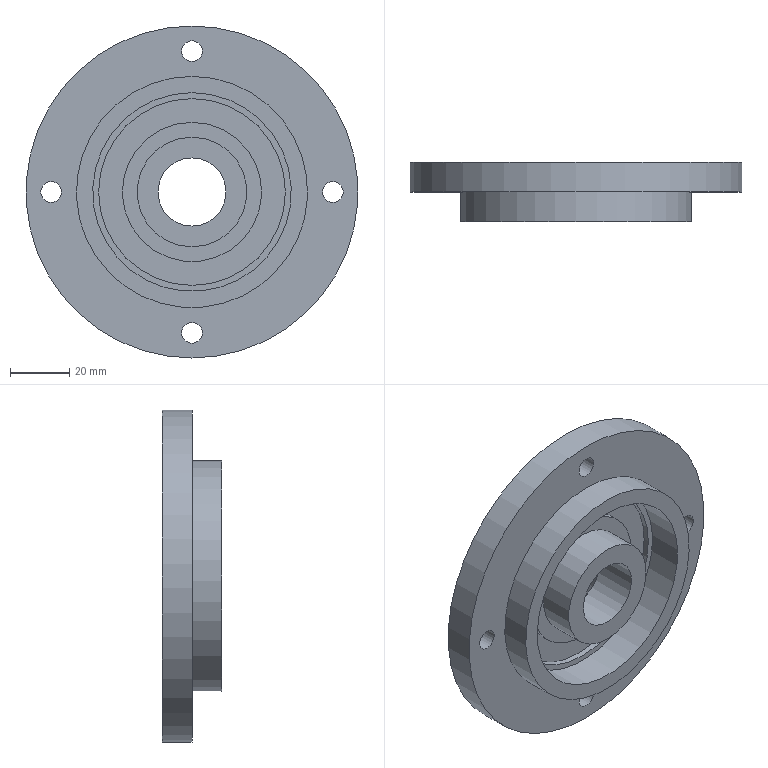Part | STEP file | Outer part of clamping device | 1 solid | 27 faces | box 112 x 20 x 112 mm | volume 101943 mm3 | cylinder 15 | plane 11 | cone 1 | commonest cylinder face diameters 7 x4 12 x4 23 x1 37 x1 47 x1 63 x1
STEP:
#1=CARTESIAN_POINT('',(0.,20.,56.));
#2=VERTEX_POINT('',#1);
#3=CARTESIAN_POINT('',(0.,20.,0.));
#4=DIRECTION('',(0.,1.,0.));
#5=DIRECTION('',(0.,0.,1.));
#6=AXIS2_PLACEMENT_3D('',#3,#4,#5);
#7=CIRCLE('',#6,56.);
#8=EDGE_CURVE('',#2,#2,#7,.T.);
#9=ORIENTED_EDGE('',*,*,#8,.T.);
#10=EDGE_LOOP('',(#9));
#11=FACE_BOUND('',#10,.T.);
#12=CARTESIAN_POINT('',(47.5,20.,6.));
#13=VERTEX_POINT('',#12);
#14=CARTESIAN_POINT('',(47.5,20.,0.));
#15=DIRECTION('',(0.,1.,0.));
#16=DIRECTION('',(0.,0.,1.));
#17=AXIS2_PLACEMENT_3D('',#14,#15,#16);
#18=CIRCLE('',#17,6.);
#19=EDGE_CURVE('',#13,#13,#18,.F.);
#20=ORIENTED_EDGE('',*,*,#19,.T.);
#21=EDGE_LOOP('',(#20));
#22=FACE_BOUND('',#21,.T.);
#23=CARTESIAN_POINT('',(-6.,20.,47.5));
#24=VERTEX_POINT('',#23);
#25=CARTESIAN_POINT('',(0.,20.,47.5));
#26=DIRECTION('',(0.,1.,0.));
#27=DIRECTION('',(-1.,0.,0.));
#28=AXIS2_PLACEMENT_3D('',#25,#26,#27);
#29=CIRCLE('',#28,6.);
#30=EDGE_CURVE('',#24,#24,#29,.F.);
#31=ORIENTED_EDGE('',*,*,#30,.T.);
#32=EDGE_LOOP('',(#31));
#33=FACE_BOUND('',#32,.T.);
#34=CARTESIAN_POINT('',(-47.5,20.,-6.));
#35=VERTEX_POINT('',#34);
#36=CARTESIAN_POINT('',(-47.5,20.,0.));
#37=DIRECTION('',(0.,1.,0.));
#38=DIRECTION('',(0.,0.,-1.));
#39=AXIS2_PLACEMENT_3D('',#36,#37,#38);
#40=CIRCLE('',#39,6.);
#41=EDGE_CURVE('',#35,#35,#40,.F.);
#42=ORIENTED_EDGE('',*,*,#41,.T.);
#43=EDGE_LOOP('',(#42));
#44=FACE_BOUND('',#43,.T.);
#45=CARTESIAN_POINT('',(0.,20.,-15.695));
#46=VERTEX_POINT('',#45);
#47=CARTESIAN_POINT('',(0.,20.,0.));
#48=DIRECTION('',(0.,1.,0.));
#49=DIRECTION('',(0.,0.,-1.));
#50=AXIS2_PLACEMENT_3D('',#47,#48,#49);
#51=CIRCLE('',#50,15.695);
#52=EDGE_CURVE('',#46,#46,#51,.F.);
#53=ORIENTED_EDGE('',*,*,#52,.T.);
#54=EDGE_LOOP('',(#53));
#55=FACE_BOUND('',#54,.T.);
#56=CARTESIAN_POINT('',(6.,20.,-47.5));
#57=VERTEX_POINT('',#56);
#58=CARTESIAN_POINT('',(0.,20.,-47.5));
#59=DIRECTION('',(0.,1.,0.));
#60=DIRECTION('',(1.,0.,0.));
#61=AXIS2_PLACEMENT_3D('',#58,#59,#60);
#62=CIRCLE('',#61,6.);
#63=EDGE_CURVE('',#57,#57,#62,.F.);
#64=ORIENTED_EDGE('',*,*,#63,.T.);
#65=EDGE_LOOP('',(#64));
#66=FACE_BOUND('',#65,.T.);
#67=CARTESIAN_POINT('',(0.,20.,0.));
#68=DIRECTION('',(0.,1.,0.));
#69=DIRECTION('',(0.,0.,1.));
#70=AXIS2_PLACEMENT_3D('',#67,#68,#69);
#71=PLANE('',#70);
#72=ADVANCED_FACE('',(#11,#22,#33,#44,#55,#66),#71,.T.);
#73=CARTESIAN_POINT('',(0.,10.,56.));
#74=VERTEX_POINT('',#73);
#75=CARTESIAN_POINT('',(0.,10.,0.));
#76=DIRECTION('',(0.,1.,0.));
#77=DIRECTION('',(0.,0.,1.));
#78=AXIS2_PLACEMENT_3D('',#75,#76,#77);
#79=CIRCLE('',#78,56.);
#80=EDGE_CURVE('',#74,#74,#79,.T.);
#81=ORIENTED_EDGE('',*,*,#80,.F.);
#82=EDGE_LOOP('',(#81));
#83=FACE_BOUND('',#82,.T.);
#84=CARTESIAN_POINT('',(47.5,10.,3.5));
#85=VERTEX_POINT('',#84);
#86=CARTESIAN_POINT('',(47.5,10.,0.));
#87=DIRECTION('',(0.,1.,0.));
#88=DIRECTION('',(0.,0.,1.));
#89=AXIS2_PLACEMENT_3D('',#86,#87,#88);
#90=CIRCLE('',#89,3.5);
#91=EDGE_CURVE('',#85,#85,#90,.T.);
#92=ORIENTED_EDGE('',*,*,#91,.T.);
#93=EDGE_LOOP('',(#92));
#94=FACE_BOUND('',#93,.T.);
#95=CARTESIAN_POINT('',(-3.5,10.,47.5));
#96=VERTEX_POINT('',#95);
#97=CARTESIAN_POINT('',(0.,10.,47.5));
#98=DIRECTION('',(0.,1.,0.));
#99=DIRECTION('',(-1.,0.,0.));
#100=AXIS2_PLACEMENT_3D('',#97,#98,#99);
#101=CIRCLE('',#100,3.5);
#102=EDGE_CURVE('',#96,#96,#101,.T.);
#103=ORIENTED_EDGE('',*,*,#102,.T.);
#104=EDGE_LOOP('',(#103));
#105=FACE_BOUND('',#104,.T.);
#106=CARTESIAN_POINT('',(-47.5,10.,-3.5));
#107=VERTEX_POINT('',#106);
#108=CARTESIAN_POINT('',(-47.5,10.,0.));
#109=DIRECTION('',(0.,1.,0.));
#110=DIRECTION('',(0.,0.,-1.));
#111=AXIS2_PLACEMENT_3D('',#108,#109,#110);
#112=CIRCLE('',#111,3.5);
#113=EDGE_CURVE('',#107,#107,#112,.T.);
#114=ORIENTED_EDGE('',*,*,#113,.T.);
#115=EDGE_LOOP('',(#114));
#116=FACE_BOUND('',#115,.T.);
#117=CARTESIAN_POINT('',(0.,10.,39.));
#118=VERTEX_POINT('',#117);
#119=CARTESIAN_POINT('',(0.,10.,0.));
#120=DIRECTION('',(0.,1.,0.));
#121=DIRECTION('',(0.,0.,1.));
#122=AXIS2_PLACEMENT_3D('',#119,#120,#121);
#123=CIRCLE('',#122,39.);
#124=EDGE_CURVE('',#118,#118,#123,.T.);
#125=ORIENTED_EDGE('',*,*,#124,.T.);
#126=EDGE_LOOP('',(#125));
#127=FACE_BOUND('',#126,.T.);
#128=CARTESIAN_POINT('',(3.5,10.,-47.5));
#129=VERTEX_POINT('',#128);
#130=CARTESIAN_POINT('',(0.,10.,-47.5));
#131=DIRECTION('',(0.,1.,0.));
#132=DIRECTION('',(1.,0.,0.));
#133=AXIS2_PLACEMENT_3D('',#130,#131,#132);
#134=CIRCLE('',#133,3.5);
#135=EDGE_CURVE('',#129,#129,#134,.T.);
#136=ORIENTED_EDGE('',*,*,#135,.T.);
#137=EDGE_LOOP('',(#136));
#138=FACE_BOUND('',#137,.T.);
#139=CARTESIAN_POINT('',(0.,10.,0.));
#140=DIRECTION('',(0.,-1.,0.));
#141=DIRECTION('',(0.,0.,1.));
#142=AXIS2_PLACEMENT_3D('',#139,#140,#141);
#143=PLANE('',#142);
#144=ADVANCED_FACE('',(#83,#94,#105,#116,#127,#138),#143,.T.);
#145=CARTESIAN_POINT('',(-47.5,15.,-3.5));
#146=VERTEX_POINT('',#145);
#147=CARTESIAN_POINT('',(-47.5,15.,0.));
#148=DIRECTION('',(0.,1.,0.));
#149=DIRECTION('',(0.,0.,-1.));
#150=AXIS2_PLACEMENT_3D('',#147,#148,#149);
#151=CIRCLE('',#150,3.5);
#152=EDGE_CURVE('',#146,#146,#151,.T.);
#153=ORIENTED_EDGE('',*,*,#152,.T.);
#154=EDGE_LOOP('',(#153));
#155=FACE_OUTER_BOUND('',#154,.T.);
#156=ORIENTED_EDGE('',*,*,#113,.F.);
#157=EDGE_LOOP('',(#156));
#158=FACE_OUTER_BOUND('',#157,.T.);
#159=CARTESIAN_POINT('',(-47.5,-20.,0.));
#160=DIRECTION('',(0.,1.,0.));
#161=DIRECTION('',(0.,0.,-1.));
#162=AXIS2_PLACEMENT_3D('',#159,#160,#161);
#163=CYLINDRICAL_SURFACE('',#162,3.5);
#164=ADVANCED_FACE('',(#155,#158),#163,.F.);
#165=ORIENTED_EDGE('',*,*,#41,.F.);
#166=EDGE_LOOP('',(#165));
#167=FACE_OUTER_BOUND('',#166,.T.);
#168=CARTESIAN_POINT('',(-47.5,15.,-6.));
#169=VERTEX_POINT('',#168);
#170=CARTESIAN_POINT('',(-47.5,15.,0.));
#171=DIRECTION('',(0.,1.,0.));
#172=DIRECTION('',(0.,0.,-1.));
#173=AXIS2_PLACEMENT_3D('',#170,#171,#172);
#174=CIRCLE('',#173,6.);
#175=EDGE_CURVE('',#169,#169,#174,.T.);
#176=ORIENTED_EDGE('',*,*,#175,.F.);
#177=EDGE_LOOP('',(#176));
#178=FACE_OUTER_BOUND('',#177,.T.);
#179=CARTESIAN_POINT('',(-47.5,15.,0.));
#180=DIRECTION('',(0.,1.,0.));
#181=DIRECTION('',(0.,0.,-1.));
#182=AXIS2_PLACEMENT_3D('',#179,#180,#181);
#183=CYLINDRICAL_SURFACE('',#182,6.);
#184=ADVANCED_FACE('',(#167,#178),#183,.F.);
#185=CARTESIAN_POINT('',(-3.5,15.,47.5));
#186=VERTEX_POINT('',#185);
#187=CARTESIAN_POINT('',(0.,15.,47.5));
#188=DIRECTION('',(0.,1.,0.));
#189=DIRECTION('',(-1.,0.,0.));
#190=AXIS2_PLACEMENT_3D('',#187,#188,#189);
#191=CIRCLE('',#190,3.5);
#192=EDGE_CURVE('',#186,#186,#191,.T.);
#193=ORIENTED_EDGE('',*,*,#192,.T.);
#194=EDGE_LOOP('',(#193));
#195=FACE_OUTER_BOUND('',#194,.T.);
#196=ORIENTED_EDGE('',*,*,#102,.F.);
#197=EDGE_LOOP('',(#196));
#198=FACE_OUTER_BOUND('',#197,.T.);
#199=CARTESIAN_POINT('',(0.,-20.,47.5));
#200=DIRECTION('',(0.,1.,0.));
#201=DIRECTION('',(-1.,0.,0.));
#202=AXIS2_PLACEMENT_3D('',#199,#200,#201);
#203=CYLINDRICAL_SURFACE('',#202,3.5);
#204=ADVANCED_FACE('',(#195,#198),#203,.F.);
#205=ORIENTED_EDGE('',*,*,#30,.F.);
#206=EDGE_LOOP('',(#205));
#207=FACE_OUTER_BOUND('',#206,.T.);
#208=CARTESIAN_POINT('',(-6.,15.,47.5));
#209=VERTEX_POINT('',#208);
#210=CARTESIAN_POINT('',(0.,15.,47.5));
#211=DIRECTION('',(0.,1.,0.));
#212=DIRECTION('',(-1.,0.,0.));
#213=AXIS2_PLACEMENT_3D('',#210,#211,#212);
#214=CIRCLE('',#213,6.);
#215=EDGE_CURVE('',#209,#209,#214,.T.);
#216=ORIENTED_EDGE('',*,*,#215,.F.);
#217=EDGE_LOOP('',(#216));
#218=FACE_OUTER_BOUND('',#217,.T.);
#219=CARTESIAN_POINT('',(0.,15.,47.5));
#220=DIRECTION('',(0.,1.,0.));
#221=DIRECTION('',(-1.,0.,0.));
#222=AXIS2_PLACEMENT_3D('',#219,#220,#221);
#223=CYLINDRICAL_SURFACE('',#222,6.);
#224=ADVANCED_FACE('',(#207,#218),#223,.F.);
#225=CARTESIAN_POINT('',(47.5,15.,3.5));
#226=VERTEX_POINT('',#225);
#227=CARTESIAN_POINT('',(47.5,15.,0.));
#228=DIRECTION('',(0.,1.,0.));
#229=DIRECTION('',(0.,0.,1.));
#230=AXIS2_PLACEMENT_3D('',#227,#228,#229);
#231=CIRCLE('',#230,3.5);
#232=EDGE_CURVE('',#226,#226,#231,.T.);
#233=ORIENTED_EDGE('',*,*,#232,.T.);
#234=EDGE_LOOP('',(#233));
#235=FACE_OUTER_BOUND('',#234,.T.);
#236=ORIENTED_EDGE('',*,*,#91,.F.);
#237=EDGE_LOOP('',(#236));
#238=FACE_OUTER_BOUND('',#237,.T.);
#239=CARTESIAN_POINT('',(47.5,-20.,0.));
#240=DIRECTION('',(0.,1.,0.));
#241=DIRECTION('',(0.,0.,1.));
#242=AXIS2_PLACEMENT_3D('',#239,#240,#241);
#243=CYLINDRICAL_SURFACE('',#242,3.5);
#244=ADVANCED_FACE('',(#235,#238),#243,.F.);
#245=ORIENTED_EDGE('',*,*,#19,.F.);
#246=EDGE_LOOP('',(#245));
#247=FACE_OUTER_BOUND('',#246,.T.);
#248=CARTESIAN_POINT('',(47.5,15.,6.));
#249=VERTEX_POINT('',#248);
#250=CARTESIAN_POINT('',(47.5,15.,0.));
#251=DIRECTION('',(0.,1.,0.));
#252=DIRECTION('',(0.,0.,1.));
#253=AXIS2_PLACEMENT_3D('',#250,#251,#252);
#254=CIRCLE('',#253,6.);
#255=EDGE_CURVE('',#249,#249,#254,.T.);
#256=ORIENTED_EDGE('',*,*,#255,.F.);
#257=EDGE_LOOP('',(#256));
#258=FACE_OUTER_BOUND('',#257,.T.);
#259=CARTESIAN_POINT('',(47.5,15.,0.));
#260=DIRECTION('',(0.,1.,0.));
#261=DIRECTION('',(0.,0.,1.));
#262=AXIS2_PLACEMENT_3D('',#259,#260,#261);
#263=CYLINDRICAL_SURFACE('',#262,6.);
#264=ADVANCED_FACE('',(#247,#258),#263,.F.);
#265=ORIENTED_EDGE('',*,*,#8,.F.);
#266=EDGE_LOOP('',(#265));
#267=FACE_OUTER_BOUND('',#266,.T.);
#268=ORIENTED_EDGE('',*,*,#80,.T.);
#269=EDGE_LOOP('',(#268));
#270=FACE_OUTER_BOUND('',#269,.T.);
#271=CARTESIAN_POINT('',(0.,10.,0.));
#272=DIRECTION('',(0.,1.,0.));
#273=DIRECTION('',(0.,0.,1.));
#274=AXIS2_PLACEMENT_3D('',#271,#272,#273);
#275=CYLINDRICAL_SURFACE('',#274,56.);
#276=ADVANCED_FACE('',(#267,#270),#275,.T.);
#277=ORIENTED_EDGE('',*,*,#52,.F.);
#278=EDGE_LOOP('',(#277));
#279=FACE_OUTER_BOUND('',#278,.T.);
#280=CARTESIAN_POINT('',(0.,15.,-11.5));
#281=VERTEX_POINT('',#280);
#282=CARTESIAN_POINT('',(0.,15.,11.5));
#283=VERTEX_POINT('',#282);
#284=CARTESIAN_POINT('',(0.,15.,0.));
#285=DIRECTION('',(0.,1.,0.));
#286=DIRECTION('',(0.,0.,-1.));
#287=AXIS2_PLACEMENT_3D('',#284,#285,#286);
#288=CIRCLE('',#287,11.5);
#289=EDGE_CURVE('',#281,#283,#288,.T.);
#290=ORIENTED_EDGE('',*,*,#289,.F.);
#291=CARTESIAN_POINT('',(0.,15.,0.));
#292=DIRECTION('',(0.,1.,0.));
#293=DIRECTION('',(0.,0.,1.));
#294=AXIS2_PLACEMENT_3D('',#291,#292,#293);
#295=CIRCLE('',#294,11.5);
#296=EDGE_CURVE('',#283,#281,#295,.T.);
#297=ORIENTED_EDGE('',*,*,#296,.F.);
#298=EDGE_LOOP('',(#290,#297));
#299=FACE_BOUND('',#298,.T.);
#300=CARTESIAN_POINT('',(0.,17.5,0.));
#301=DIRECTION('',(0.,1.,0.));
#302=DIRECTION('',(0.,0.,-1.));
#303=AXIS2_PLACEMENT_3D('',#300,#301,#302);
#304=CONICAL_SURFACE('',#303,13.598,0.6981);
#305=ADVANCED_FACE('',(#279,#299),#304,.F.);
#306=ORIENTED_EDGE('',*,*,#63,.F.);
#307=EDGE_LOOP('',(#306));
#308=FACE_OUTER_BOUND('',#307,.T.);
#309=CARTESIAN_POINT('',(6.,15.,-47.5));
#310=VERTEX_POINT('',#309);
#311=CARTESIAN_POINT('',(0.,15.,-47.5));
#312=DIRECTION('',(0.,1.,0.));
#313=DIRECTION('',(1.,0.,0.));
#314=AXIS2_PLACEMENT_3D('',#311,#312,#313);
#315=CIRCLE('',#314,6.);
#316=EDGE_CURVE('',#310,#310,#315,.T.);
#317=ORIENTED_EDGE('',*,*,#316,.F.);
#318=EDGE_LOOP('',(#317));
#319=FACE_OUTER_BOUND('',#318,.T.);
#320=CARTESIAN_POINT('',(0.,15.,-47.5));
#321=DIRECTION('',(0.,1.,0.));
#322=DIRECTION('',(1.,0.,0.));
#323=AXIS2_PLACEMENT_3D('',#320,#321,#322);
#324=CYLINDRICAL_SURFACE('',#323,6.);
#325=ADVANCED_FACE('',(#308,#319),#324,.F.);
#326=ORIENTED_EDGE('',*,*,#124,.F.);
#327=EDGE_LOOP('',(#326));
#328=FACE_OUTER_BOUND('',#327,.T.);
#329=CARTESIAN_POINT('',(0.,0.,39.));
#330=VERTEX_POINT('',#329);
#331=CARTESIAN_POINT('',(0.,0.,0.));
#332=DIRECTION('',(0.,1.,0.));
#333=DIRECTION('',(0.,0.,1.));
#334=AXIS2_PLACEMENT_3D('',#331,#332,#333);
#335=CIRCLE('',#334,39.);
#336=EDGE_CURVE('',#330,#330,#335,.T.);
#337=ORIENTED_EDGE('',*,*,#336,.T.);
#338=EDGE_LOOP('',(#337));
#339=FACE_OUTER_BOUND('',#338,.T.);
#340=CARTESIAN_POINT('',(0.,0.,0.));
#341=DIRECTION('',(0.,1.,0.));
#342=DIRECTION('',(0.,0.,1.));
#343=AXIS2_PLACEMENT_3D('',#340,#341,#342);
#344=CYLINDRICAL_SURFACE('',#343,39.);
#345=ADVANCED_FACE('',(#328,#339),#344,.T.);
#346=CARTESIAN_POINT('',(3.5,15.,-47.5));
#347=VERTEX_POINT('',#346);
#348=CARTESIAN_POINT('',(0.,15.,-47.5));
#349=DIRECTION('',(0.,1.,0.));
#350=DIRECTION('',(1.,0.,0.));
#351=AXIS2_PLACEMENT_3D('',#348,#349,#350);
#352=CIRCLE('',#351,3.5);
#353=EDGE_CURVE('',#347,#347,#352,.T.);
#354=ORIENTED_EDGE('',*,*,#353,.T.);
#355=EDGE_LOOP('',(#354));
#356=FACE_OUTER_BOUND('',#355,.T.);
#357=ORIENTED_EDGE('',*,*,#135,.F.);
#358=EDGE_LOOP('',(#357));
#359=FACE_OUTER_BOUND('',#358,.T.);
#360=CARTESIAN_POINT('',(0.,-20.,-47.5));
#361=DIRECTION('',(0.,1.,0.));
#362=DIRECTION('',(1.,0.,0.));
#363=AXIS2_PLACEMENT_3D('',#360,#361,#362);
#364=CYLINDRICAL_SURFACE('',#363,3.5);
#365=ADVANCED_FACE('',(#356,#359),#364,.F.);
#366=ORIENTED_EDGE('',*,*,#175,.T.);
#367=EDGE_LOOP('',(#366));
#368=FACE_BOUND('',#367,.T.);
#369=ORIENTED_EDGE('',*,*,#152,.F.);
#370=EDGE_LOOP('',(#369));
#371=FACE_BOUND('',#370,.T.);
#372=CARTESIAN_POINT('',(-47.5,15.,0.));
#373=DIRECTION('',(0.,-1.,0.));
#374=DIRECTION('',(0.,0.,-1.));
#375=AXIS2_PLACEMENT_3D('',#372,#373,#374);
#376=PLANE('',#375);
#377=ADVANCED_FACE('',(#368,#371),#376,.F.);
#378=ORIENTED_EDGE('',*,*,#215,.T.);
#379=EDGE_LOOP('',(#378));
#380=FACE_BOUND('',#379,.T.);
#381=ORIENTED_EDGE('',*,*,#192,.F.);
#382=EDGE_LOOP('',(#381));
#383=FACE_BOUND('',#382,.T.);
#384=CARTESIAN_POINT('',(0.,15.,47.5));
#385=DIRECTION('',(0.,-1.,0.));
#386=DIRECTION('',(-1.,0.,0.));
#387=AXIS2_PLACEMENT_3D('',#384,#385,#386);
#388=PLANE('',#387);
#389=ADVANCED_FACE('',(#380,#383),#388,.F.);
#390=ORIENTED_EDGE('',*,*,#255,.T.);
#391=EDGE_LOOP('',(#390));
#392=FACE_BOUND('',#391,.T.);
#393=ORIENTED_EDGE('',*,*,#232,.F.);
#394=EDGE_LOOP('',(#393));
#395=FACE_BOUND('',#394,.T.);
#396=CARTESIAN_POINT('',(47.5,15.,0.));
#397=DIRECTION('',(0.,-1.,0.));
#398=DIRECTION('',(0.,0.,1.));
#399=AXIS2_PLACEMENT_3D('',#396,#397,#398);
#400=PLANE('',#399);
#401=ADVANCED_FACE('',(#392,#395),#400,.F.);
#402=ORIENTED_EDGE('',*,*,#296,.T.);
#403=ORIENTED_EDGE('',*,*,#289,.T.);
#404=EDGE_LOOP('',(#402,#403));
#405=FACE_BOUND('',#404,.T.);
#406=CARTESIAN_POINT('',(0.,0.,11.5));
#407=VERTEX_POINT('',#406);
#408=CARTESIAN_POINT('',(0.,0.,0.));
#409=DIRECTION('',(0.,1.,0.));
#410=DIRECTION('',(0.,0.,1.));
#411=AXIS2_PLACEMENT_3D('',#408,#409,#410);
#412=CIRCLE('',#411,11.5);
#413=EDGE_CURVE('',#407,#407,#412,.T.);
#414=ORIENTED_EDGE('',*,*,#413,.F.);
#415=EDGE_LOOP('',(#414));
#416=FACE_OUTER_BOUND('',#415,.T.);
#417=CARTESIAN_POINT('',(0.,20.,0.));
#418=DIRECTION('',(0.,1.,0.));
#419=DIRECTION('',(0.,0.,1.));
#420=AXIS2_PLACEMENT_3D('',#417,#418,#419);
#421=CYLINDRICAL_SURFACE('',#420,11.5);
#422=ADVANCED_FACE('',(#405,#416),#421,.F.);
#423=ORIENTED_EDGE('',*,*,#316,.T.);
#424=EDGE_LOOP('',(#423));
#425=FACE_BOUND('',#424,.T.);
#426=ORIENTED_EDGE('',*,*,#353,.F.);
#427=EDGE_LOOP('',(#426));
#428=FACE_BOUND('',#427,.T.);
#429=CARTESIAN_POINT('',(0.,15.,-47.5));
#430=DIRECTION('',(0.,-1.,0.));
#431=DIRECTION('',(1.,0.,0.));
#432=AXIS2_PLACEMENT_3D('',#429,#430,#431);
#433=PLANE('',#432);
#434=ADVANCED_FACE('',(#425,#428),#433,.F.);
#435=ORIENTED_EDGE('',*,*,#336,.F.);
#436=EDGE_LOOP('',(#435));
#437=FACE_BOUND('',#436,.T.);
#438=CARTESIAN_POINT('',(0.,0.,33.5));
#439=VERTEX_POINT('',#438);
#440=CARTESIAN_POINT('',(0.,0.,0.));
#441=DIRECTION('',(0.,1.,0.));
#442=DIRECTION('',(0.,0.,1.));
#443=AXIS2_PLACEMENT_3D('',#440,#441,#442);
#444=CIRCLE('',#443,33.5);
#445=EDGE_CURVE('',#439,#439,#444,.T.);
#446=ORIENTED_EDGE('',*,*,#445,.T.);
#447=EDGE_LOOP('',(#446));
#448=FACE_BOUND('',#447,.T.);
#449=CARTESIAN_POINT('',(0.,0.,0.));
#450=DIRECTION('',(0.,-1.,0.));
#451=DIRECTION('',(0.,0.,1.));
#452=AXIS2_PLACEMENT_3D('',#449,#450,#451);
#453=PLANE('',#452);
#454=ADVANCED_FACE('',(#437,#448),#453,.T.);
#455=CARTESIAN_POINT('',(0.,0.,18.5));
#456=VERTEX_POINT('',#455);
#457=CARTESIAN_POINT('',(0.,0.,0.));
#458=DIRECTION('',(0.,1.,0.));
#459=DIRECTION('',(0.,0.,1.));
#460=AXIS2_PLACEMENT_3D('',#457,#458,#459);
#461=CIRCLE('',#460,18.5);
#462=EDGE_CURVE('',#456,#456,#461,.T.);
#463=ORIENTED_EDGE('',*,*,#462,.F.);
#464=EDGE_LOOP('',(#463));
#465=FACE_BOUND('',#464,.T.);
#466=ORIENTED_EDGE('',*,*,#413,.T.);
#467=EDGE_LOOP('',(#466));
#468=FACE_BOUND('',#467,.T.);
#469=CARTESIAN_POINT('',(0.,0.,0.));
#470=DIRECTION('',(0.,-1.,0.));
#471=DIRECTION('',(0.,0.,1.));
#472=AXIS2_PLACEMENT_3D('',#469,#470,#471);
#473=PLANE('',#472);
#474=ADVANCED_FACE('',(#465,#468),#473,.T.);
#475=CARTESIAN_POINT('',(0.,12.,33.5));
#476=VERTEX_POINT('',#475);
#477=CARTESIAN_POINT('',(0.,12.,0.));
#478=DIRECTION('',(0.,1.,0.));
#479=DIRECTION('',(0.,0.,1.));
#480=AXIS2_PLACEMENT_3D('',#477,#478,#479);
#481=CIRCLE('',#480,33.5);
#482=EDGE_CURVE('',#476,#476,#481,.T.);
#483=ORIENTED_EDGE('',*,*,#482,.T.);
#484=EDGE_LOOP('',(#483));
#485=FACE_OUTER_BOUND('',#484,.T.);
#486=ORIENTED_EDGE('',*,*,#445,.F.);
#487=EDGE_LOOP('',(#486));
#488=FACE_OUTER_BOUND('',#487,.T.);
#489=CARTESIAN_POINT('',(0.,12.,0.));
#490=DIRECTION('',(0.,1.,0.));
#491=DIRECTION('',(0.,0.,1.));
#492=AXIS2_PLACEMENT_3D('',#489,#490,#491);
#493=CYLINDRICAL_SURFACE('',#492,33.5);
#494=ADVANCED_FACE('',(#485,#488),#493,.F.);
#495=CARTESIAN_POINT('',(0.,12.,18.5));
#496=VERTEX_POINT('',#495);
#497=CARTESIAN_POINT('',(0.,12.,0.));
#498=DIRECTION('',(0.,1.,0.));
#499=DIRECTION('',(0.,0.,1.));
#500=AXIS2_PLACEMENT_3D('',#497,#498,#499);
#501=CIRCLE('',#500,18.5);
#502=EDGE_CURVE('',#496,#496,#501,.T.);
#503=ORIENTED_EDGE('',*,*,#502,.F.);
#504=EDGE_LOOP('',(#503));
#505=FACE_OUTER_BOUND('',#504,.T.);
#506=ORIENTED_EDGE('',*,*,#462,.T.);
#507=EDGE_LOOP('',(#506));
#508=FACE_OUTER_BOUND('',#507,.T.);
#509=CARTESIAN_POINT('',(0.,0.,0.));
#510=DIRECTION('',(0.,1.,0.));
#511=DIRECTION('',(0.,0.,1.));
#512=AXIS2_PLACEMENT_3D('',#509,#510,#511);
#513=CYLINDRICAL_SURFACE('',#512,18.5);
#514=ADVANCED_FACE('',(#505,#508),#513,.T.);
#515=ORIENTED_EDGE('',*,*,#482,.F.);
#516=EDGE_LOOP('',(#515));
#517=FACE_BOUND('',#516,.T.);
#518=CARTESIAN_POINT('',(0.,12.,31.5));
#519=VERTEX_POINT('',#518);
#520=CARTESIAN_POINT('',(0.,12.,0.));
#521=DIRECTION('',(0.,1.,0.));
#522=DIRECTION('',(0.,0.,1.));
#523=AXIS2_PLACEMENT_3D('',#520,#521,#522);
#524=CIRCLE('',#523,31.5);
#525=EDGE_CURVE('',#519,#519,#524,.T.);
#526=ORIENTED_EDGE('',*,*,#525,.T.);
#527=EDGE_LOOP('',(#526));
#528=FACE_BOUND('',#527,.T.);
#529=CARTESIAN_POINT('',(0.,12.,0.));
#530=DIRECTION('',(0.,-1.,0.));
#531=DIRECTION('',(0.,0.,1.));
#532=AXIS2_PLACEMENT_3D('',#529,#530,#531);
#533=PLANE('',#532);
#534=ADVANCED_FACE('',(#517,#528),#533,.T.);
#535=CARTESIAN_POINT('',(0.,12.,23.5));
#536=VERTEX_POINT('',#535);
#537=CARTESIAN_POINT('',(0.,12.,0.));
#538=DIRECTION('',(0.,1.,0.));
#539=DIRECTION('',(0.,0.,1.));
#540=AXIS2_PLACEMENT_3D('',#537,#538,#539);
#541=CIRCLE('',#540,23.5);
#542=EDGE_CURVE('',#536,#536,#541,.T.);
#543=ORIENTED_EDGE('',*,*,#542,.F.);
#544=EDGE_LOOP('',(#543));
#545=FACE_BOUND('',#544,.T.);
#546=ORIENTED_EDGE('',*,*,#502,.T.);
#547=EDGE_LOOP('',(#546));
#548=FACE_BOUND('',#547,.T.);
#549=CARTESIAN_POINT('',(0.,12.,0.));
#550=DIRECTION('',(0.,-1.,0.));
#551=DIRECTION('',(0.,0.,1.));
#552=AXIS2_PLACEMENT_3D('',#549,#550,#551);
#553=PLANE('',#552);
#554=ADVANCED_FACE('',(#545,#548),#553,.T.);
#555=CARTESIAN_POINT('',(0.,14.,31.5));
#556=VERTEX_POINT('',#555);
#557=CARTESIAN_POINT('',(0.,14.,0.));
#558=DIRECTION('',(0.,1.,0.));
#559=DIRECTION('',(0.,0.,1.));
#560=AXIS2_PLACEMENT_3D('',#557,#558,#559);
#561=CIRCLE('',#560,31.5);
#562=EDGE_CURVE('',#556,#556,#561,.T.);
#563=ORIENTED_EDGE('',*,*,#562,.T.);
#564=EDGE_LOOP('',(#563));
#565=FACE_OUTER_BOUND('',#564,.T.);
#566=ORIENTED_EDGE('',*,*,#525,.F.);
#567=EDGE_LOOP('',(#566));
#568=FACE_OUTER_BOUND('',#567,.T.);
#569=CARTESIAN_POINT('',(0.,14.,0.));
#570=DIRECTION('',(0.,1.,0.));
#571=DIRECTION('',(0.,0.,1.));
#572=AXIS2_PLACEMENT_3D('',#569,#570,#571);
#573=CYLINDRICAL_SURFACE('',#572,31.5);
#574=ADVANCED_FACE('',(#565,#568),#573,.F.);
#575=CARTESIAN_POINT('',(0.,14.,23.5));
#576=VERTEX_POINT('',#575);
#577=CARTESIAN_POINT('',(0.,14.,0.));
#578=DIRECTION('',(0.,1.,0.));
#579=DIRECTION('',(0.,0.,1.));
#580=AXIS2_PLACEMENT_3D('',#577,#578,#579);
#581=CIRCLE('',#580,23.5);
#582=EDGE_CURVE('',#576,#576,#581,.T.);
#583=ORIENTED_EDGE('',*,*,#582,.F.);
#584=EDGE_LOOP('',(#583));
#585=FACE_OUTER_BOUND('',#584,.T.);
#586=ORIENTED_EDGE('',*,*,#542,.T.);
#587=EDGE_LOOP('',(#586));
#588=FACE_OUTER_BOUND('',#587,.T.);
#589=CARTESIAN_POINT('',(0.,12.,0.));
#590=DIRECTION('',(0.,1.,0.));
#591=DIRECTION('',(0.,0.,1.));
#592=AXIS2_PLACEMENT_3D('',#589,#590,#591);
#593=CYLINDRICAL_SURFACE('',#592,23.5);
#594=ADVANCED_FACE('',(#585,#588),#593,.T.);
#595=ORIENTED_EDGE('',*,*,#562,.F.);
#596=EDGE_LOOP('',(#595));
#597=FACE_BOUND('',#596,.T.);
#598=ORIENTED_EDGE('',*,*,#582,.T.);
#599=EDGE_LOOP('',(#598));
#600=FACE_BOUND('',#599,.T.);
#601=CARTESIAN_POINT('',(0.,14.,0.));
#602=DIRECTION('',(0.,-1.,0.));
#603=DIRECTION('',(0.,0.,1.));
#604=AXIS2_PLACEMENT_3D('',#601,#602,#603);
#605=PLANE('',#604);
#606=ADVANCED_FACE('',(#597,#600),#605,.T.);
#607=CLOSED_SHELL('',(#72,#144,#164,#184,#204,#224,#244,#264,#276,#305,#325,#345,#365,#377,#389,#401,#422,#434,#454,#474,#494,#514,#534,#554,#574,#594,#606));
#608=MANIFOLD_SOLID_BREP('',#607);
#609=(LENGTH_UNIT()NAMED_UNIT(*)SI_UNIT(.MILLI.,.METRE.));
#610=UNCERTAINTY_MEASURE_WITH_UNIT(LENGTH_MEASURE(0.00001),#609,'','');
#611=(NAMED_UNIT(*)PLANE_ANGLE_UNIT()SI_UNIT($,.RADIAN.));
#612=(NAMED_UNIT(*)SI_UNIT($,.STERADIAN.)SOLID_ANGLE_UNIT());
#613=(GEOMETRIC_REPRESENTATION_CONTEXT(3)GLOBAL_UNCERTAINTY_ASSIGNED_CONTEXT((#610))GLOBAL_UNIT_ASSIGNED_CONTEXT((#609,#611,#612))REPRESENTATION_CONTEXT('',''));
#614=ADVANCED_BREP_SHAPE_REPRESENTATION('',(#608),#613);